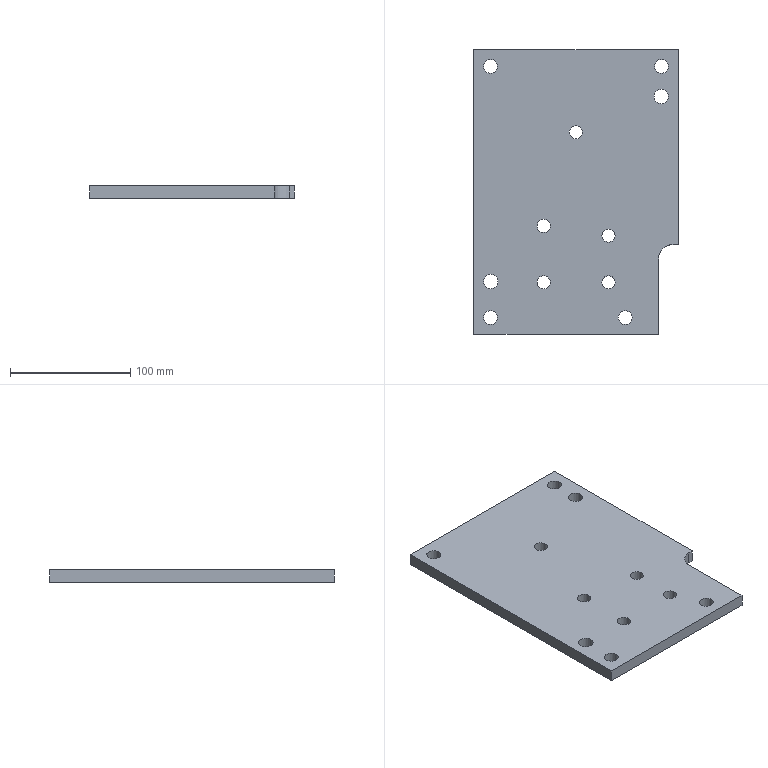Part | STEP file | lll_id2994_x_t | 1 solid | 20 faces | box 170 x 237 x 10 mm | volume 379901 mm3 | cylinder 12 | plane 8 | commonest cylinder face diameters 11 x5 11.509 x4 12 x2 24 x1
STEP:
#1=CARTESIAN_POINT('',(3581.734,202.95,92.5));
#2=VERTEX_POINT('',#1);
#3=CARTESIAN_POINT('',(3587.234,202.95,92.5));
#4=DIRECTION('',(0.,0.,-1.));
#5=DIRECTION('',(-1.,0.,0.));
#6=AXIS2_PLACEMENT_3D('',#3,#4,#5);
#7=CIRCLE('',#6,5.5);
#8=EDGE_CURVE('',#2,#2,#7,.T.);
#9=ORIENTED_EDGE('',*,*,#8,.F.);
#10=EDGE_LOOP('',(#9));
#11=FACE_BOUND('',#10,.T.);
#12=CARTESIAN_POINT('',(3608.779,117.031,92.5));
#13=VERTEX_POINT('',#12);
#14=CARTESIAN_POINT('',(3614.279,117.031,92.5));
#15=DIRECTION('',(0.,0.,-1.));
#16=DIRECTION('',(-1.,0.,0.));
#17=AXIS2_PLACEMENT_3D('',#14,#15,#16);
#18=CIRCLE('',#17,5.5);
#19=EDGE_CURVE('',#13,#13,#18,.T.);
#20=ORIENTED_EDGE('',*,*,#19,.F.);
#21=EDGE_LOOP('',(#20));
#22=FACE_BOUND('',#21,.T.);
#23=CARTESIAN_POINT('',(3554.876,78.05,92.5));
#24=VERTEX_POINT('',#23);
#25=CARTESIAN_POINT('',(3560.376,78.05,92.5));
#26=DIRECTION('',(0.,0.,-1.));
#27=DIRECTION('',(-1.,0.,0.));
#28=AXIS2_PLACEMENT_3D('',#25,#26,#27);
#29=CIRCLE('',#28,5.5);
#30=EDGE_CURVE('',#24,#24,#29,.T.);
#31=ORIENTED_EDGE('',*,*,#30,.F.);
#32=EDGE_LOOP('',(#31));
#33=FACE_BOUND('',#32,.T.);
#34=CARTESIAN_POINT('',(3510.243,78.803,92.5));
#35=VERTEX_POINT('',#34);
#36=CARTESIAN_POINT('',(3516.243,78.803,92.5));
#37=DIRECTION('',(0.,0.,1.));
#38=DIRECTION('',(-1.,0.,0.));
#39=AXIS2_PLACEMENT_3D('',#36,#37,#38);
#40=CIRCLE('',#39,6.);
#41=EDGE_CURVE('',#35,#35,#40,.T.);
#42=ORIENTED_EDGE('',*,*,#41,.T.);
#43=EDGE_LOOP('',(#42));
#44=FACE_BOUND('',#43,.T.);
#45=CARTESIAN_POINT('',(3622.489,48.803,92.5));
#46=VERTEX_POINT('',#45);
#47=CARTESIAN_POINT('',(3628.243,48.803,92.5));
#48=DIRECTION('',(0.,0.,1.));
#49=DIRECTION('',(-1.,0.,0.));
#50=AXIS2_PLACEMENT_3D('',#47,#48,#49);
#51=CIRCLE('',#50,5.755);
#52=EDGE_CURVE('',#46,#46,#51,.T.);
#53=ORIENTED_EDGE('',*,*,#52,.T.);
#54=EDGE_LOOP('',(#53));
#55=FACE_BOUND('',#54,.T.);
#56=CARTESIAN_POINT('',(3510.489,48.803,92.5));
#57=VERTEX_POINT('',#56);
#58=CARTESIAN_POINT('',(3516.243,48.803,92.5));
#59=DIRECTION('',(0.,0.,1.));
#60=DIRECTION('',(-1.,0.,0.));
#61=AXIS2_PLACEMENT_3D('',#58,#59,#60);
#62=CIRCLE('',#61,5.755);
#63=EDGE_CURVE('',#57,#57,#62,.T.);
#64=ORIENTED_EDGE('',*,*,#63,.T.);
#65=EDGE_LOOP('',(#64));
#66=FACE_BOUND('',#65,.T.);
#67=CARTESIAN_POINT('',(3652.489,257.803,92.5));
#68=VERTEX_POINT('',#67);
#69=CARTESIAN_POINT('',(3658.243,257.803,92.5));
#70=DIRECTION('',(0.,0.,1.));
#71=DIRECTION('',(-1.,0.,0.));
#72=AXIS2_PLACEMENT_3D('',#69,#70,#71);
#73=CIRCLE('',#72,5.755);
#74=EDGE_CURVE('',#68,#68,#73,.T.);
#75=ORIENTED_EDGE('',*,*,#74,.T.);
#76=EDGE_LOOP('',(#75));
#77=FACE_BOUND('',#76,.T.);
#78=CARTESIAN_POINT('',(3510.489,257.803,92.5));
#79=VERTEX_POINT('',#78);
#80=CARTESIAN_POINT('',(3516.243,257.803,92.5));
#81=DIRECTION('',(0.,0.,1.));
#82=DIRECTION('',(-1.,0.,0.));
#83=AXIS2_PLACEMENT_3D('',#80,#81,#82);
#84=CIRCLE('',#83,5.755);
#85=EDGE_CURVE('',#79,#79,#84,.T.);
#86=ORIENTED_EDGE('',*,*,#85,.T.);
#87=EDGE_LOOP('',(#86));
#88=FACE_BOUND('',#87,.T.);
#89=CARTESIAN_POINT('',(3652.243,232.803,92.5));
#90=VERTEX_POINT('',#89);
#91=CARTESIAN_POINT('',(3658.243,232.803,92.5));
#92=DIRECTION('',(0.,0.,1.));
#93=DIRECTION('',(-1.,0.,0.));
#94=AXIS2_PLACEMENT_3D('',#91,#92,#93);
#95=CIRCLE('',#94,6.);
#96=EDGE_CURVE('',#90,#90,#95,.T.);
#97=ORIENTED_EDGE('',*,*,#96,.T.);
#98=EDGE_LOOP('',(#97));
#99=FACE_BOUND('',#98,.T.);
#100=CARTESIAN_POINT('',(3672.243,109.5,92.5));
#101=VERTEX_POINT('',#100);
#102=CARTESIAN_POINT('',(3668.,109.5,92.5));
#103=VERTEX_POINT('',#102);
#104=CARTESIAN_POINT('',(3700.5,109.5,92.5));
#105=DIRECTION('',(-1.,0.,0.));
#106=VECTOR('',#105,1.);
#107=LINE('',#104,#106);
#108=EDGE_CURVE('',#101,#103,#107,.T.);
#109=ORIENTED_EDGE('',*,*,#108,.T.);
#110=CARTESIAN_POINT('',(3656.,97.5,92.5));
#111=VERTEX_POINT('',#110);
#112=CARTESIAN_POINT('',(3668.,97.5,92.5));
#113=DIRECTION('',(0.,0.,1.));
#114=DIRECTION('',(-1.,0.,0.));
#115=AXIS2_PLACEMENT_3D('',#112,#113,#114);
#116=CIRCLE('',#115,12.);
#117=EDGE_CURVE('',#103,#111,#116,.T.);
#118=ORIENTED_EDGE('',*,*,#117,.T.);
#119=CARTESIAN_POINT('',(3656.,34.803,92.5));
#120=VERTEX_POINT('',#119);
#121=CARTESIAN_POINT('',(3656.,0.00007612,92.5));
#122=DIRECTION('',(0.,-1.,0.));
#123=VECTOR('',#122,1.);
#124=LINE('',#121,#123);
#125=EDGE_CURVE('',#111,#120,#124,.T.);
#126=ORIENTED_EDGE('',*,*,#125,.T.);
#127=CARTESIAN_POINT('',(3502.243,34.803,92.5));
#128=VERTEX_POINT('',#127);
#129=CARTESIAN_POINT('',(3587.243,34.803,92.5));
#130=DIRECTION('',(1.,0.,0.));
#131=VECTOR('',#130,1.);
#132=LINE('',#129,#131);
#133=EDGE_CURVE('',#128,#120,#132,.T.);
#134=ORIENTED_EDGE('',*,*,#133,.F.);
#135=CARTESIAN_POINT('',(3502.243,271.803,92.5));
#136=VERTEX_POINT('',#135);
#137=CARTESIAN_POINT('',(3502.243,156.803,92.5));
#138=DIRECTION('',(0.,-1.,0.));
#139=VECTOR('',#138,1.);
#140=LINE('',#137,#139);
#141=EDGE_CURVE('',#136,#128,#140,.T.);
#142=ORIENTED_EDGE('',*,*,#141,.F.);
#143=CARTESIAN_POINT('',(3672.243,271.803,92.5));
#144=VERTEX_POINT('',#143);
#145=CARTESIAN_POINT('',(3587.243,271.803,92.5));
#146=DIRECTION('',(-1.,0.,0.));
#147=VECTOR('',#146,1.);
#148=LINE('',#145,#147);
#149=EDGE_CURVE('',#144,#136,#148,.T.);
#150=ORIENTED_EDGE('',*,*,#149,.F.);
#151=CARTESIAN_POINT('',(3672.243,156.803,92.5));
#152=DIRECTION('',(0.,1.,0.));
#153=VECTOR('',#152,1.);
#154=LINE('',#151,#153);
#155=EDGE_CURVE('',#101,#144,#154,.T.);
#156=ORIENTED_EDGE('',*,*,#155,.F.);
#157=EDGE_LOOP('',(#109,#118,#126,#134,#142,#150,#156));
#158=FACE_BOUND('',#157,.T.);
#159=CARTESIAN_POINT('',(3608.779,78.031,92.5));
#160=VERTEX_POINT('',#159);
#161=CARTESIAN_POINT('',(3614.279,78.031,92.5));
#162=DIRECTION('',(0.,0.,-1.));
#163=DIRECTION('',(-1.,0.,0.));
#164=AXIS2_PLACEMENT_3D('',#161,#162,#163);
#165=CIRCLE('',#164,5.5);
#166=EDGE_CURVE('',#160,#160,#165,.T.);
#167=ORIENTED_EDGE('',*,*,#166,.F.);
#168=EDGE_LOOP('',(#167));
#169=FACE_BOUND('',#168,.T.);
#170=CARTESIAN_POINT('',(3554.876,125.05,92.5));
#171=VERTEX_POINT('',#170);
#172=CARTESIAN_POINT('',(3560.376,125.05,92.5));
#173=DIRECTION('',(0.,0.,1.));
#174=DIRECTION('',(-1.,0.,0.));
#175=AXIS2_PLACEMENT_3D('',#172,#173,#174);
#176=CIRCLE('',#175,5.5);
#177=EDGE_CURVE('',#171,#171,#176,.T.);
#178=ORIENTED_EDGE('',*,*,#177,.T.);
#179=EDGE_LOOP('',(#178));
#180=FACE_BOUND('',#179,.T.);
#181=CARTESIAN_POINT('',(3587.243,156.803,92.5));
#182=DIRECTION('',(0.,0.,-1.));
#183=DIRECTION('',(1.,0.,0.));
#184=AXIS2_PLACEMENT_3D('',#181,#182,#183);
#185=PLANE('',#184);
#186=ADVANCED_FACE('',(#11,#22,#33,#44,#55,#66,#77,#88,#99,#158,#169,#180),#185,.T.);
#187=CARTESIAN_POINT('',(3581.734,202.95,102.5));
#188=VERTEX_POINT('',#187);
#189=CARTESIAN_POINT('',(3587.234,202.95,102.5));
#190=DIRECTION('',(0.,0.,-1.));
#191=DIRECTION('',(-1.,0.,0.));
#192=AXIS2_PLACEMENT_3D('',#189,#190,#191);
#193=CIRCLE('',#192,5.5);
#194=EDGE_CURVE('',#188,#188,#193,.T.);
#195=ORIENTED_EDGE('',*,*,#194,.T.);
#196=EDGE_LOOP('',(#195));
#197=FACE_BOUND('',#196,.T.);
#198=CARTESIAN_POINT('',(3608.779,117.031,102.5));
#199=VERTEX_POINT('',#198);
#200=CARTESIAN_POINT('',(3614.279,117.031,102.5));
#201=DIRECTION('',(0.,0.,-1.));
#202=DIRECTION('',(-1.,0.,0.));
#203=AXIS2_PLACEMENT_3D('',#200,#201,#202);
#204=CIRCLE('',#203,5.5);
#205=EDGE_CURVE('',#199,#199,#204,.T.);
#206=ORIENTED_EDGE('',*,*,#205,.T.);
#207=EDGE_LOOP('',(#206));
#208=FACE_BOUND('',#207,.T.);
#209=CARTESIAN_POINT('',(3554.876,78.05,102.5));
#210=VERTEX_POINT('',#209);
#211=CARTESIAN_POINT('',(3560.376,78.05,102.5));
#212=DIRECTION('',(0.,0.,-1.));
#213=DIRECTION('',(-1.,0.,0.));
#214=AXIS2_PLACEMENT_3D('',#211,#212,#213);
#215=CIRCLE('',#214,5.5);
#216=EDGE_CURVE('',#210,#210,#215,.T.);
#217=ORIENTED_EDGE('',*,*,#216,.T.);
#218=EDGE_LOOP('',(#217));
#219=FACE_BOUND('',#218,.T.);
#220=CARTESIAN_POINT('',(3652.489,257.803,102.5));
#221=VERTEX_POINT('',#220);
#222=CARTESIAN_POINT('',(3658.243,257.803,102.5));
#223=DIRECTION('',(0.,0.,1.));
#224=DIRECTION('',(-1.,0.,0.));
#225=AXIS2_PLACEMENT_3D('',#222,#223,#224);
#226=CIRCLE('',#225,5.755);
#227=EDGE_CURVE('',#221,#221,#226,.T.);
#228=ORIENTED_EDGE('',*,*,#227,.F.);
#229=EDGE_LOOP('',(#228));
#230=FACE_BOUND('',#229,.T.);
#231=CARTESIAN_POINT('',(3510.489,257.803,102.5));
#232=VERTEX_POINT('',#231);
#233=CARTESIAN_POINT('',(3516.243,257.803,102.5));
#234=DIRECTION('',(0.,0.,-1.));
#235=DIRECTION('',(-1.,0.,0.));
#236=AXIS2_PLACEMENT_3D('',#233,#234,#235);
#237=CIRCLE('',#236,5.755);
#238=EDGE_CURVE('',#232,#232,#237,.T.);
#239=ORIENTED_EDGE('',*,*,#238,.T.);
#240=EDGE_LOOP('',(#239));
#241=FACE_BOUND('',#240,.T.);
#242=CARTESIAN_POINT('',(3652.243,232.803,102.5));
#243=VERTEX_POINT('',#242);
#244=CARTESIAN_POINT('',(3658.243,232.803,102.5));
#245=DIRECTION('',(0.,0.,-1.));
#246=DIRECTION('',(-1.,0.,0.));
#247=AXIS2_PLACEMENT_3D('',#244,#245,#246);
#248=CIRCLE('',#247,6.);
#249=EDGE_CURVE('',#243,#243,#248,.T.);
#250=ORIENTED_EDGE('',*,*,#249,.T.);
#251=EDGE_LOOP('',(#250));
#252=FACE_BOUND('',#251,.T.);
#253=CARTESIAN_POINT('',(3502.243,271.803,102.5));
#254=VERTEX_POINT('',#253);
#255=CARTESIAN_POINT('',(3672.243,271.803,102.5));
#256=VERTEX_POINT('',#255);
#257=CARTESIAN_POINT('',(3587.243,271.803,102.5));
#258=DIRECTION('',(1.,0.,0.));
#259=VECTOR('',#258,1.);
#260=LINE('',#257,#259);
#261=EDGE_CURVE('',#254,#256,#260,.T.);
#262=ORIENTED_EDGE('',*,*,#261,.F.);
#263=CARTESIAN_POINT('',(3502.243,34.803,102.5));
#264=VERTEX_POINT('',#263);
#265=CARTESIAN_POINT('',(3502.243,156.803,102.5));
#266=DIRECTION('',(0.,1.,0.));
#267=VECTOR('',#266,1.);
#268=LINE('',#265,#267);
#269=EDGE_CURVE('',#264,#254,#268,.T.);
#270=ORIENTED_EDGE('',*,*,#269,.F.);
#271=CARTESIAN_POINT('',(3656.,34.803,102.5));
#272=VERTEX_POINT('',#271);
#273=CARTESIAN_POINT('',(3587.243,34.803,102.5));
#274=DIRECTION('',(-1.,0.,0.));
#275=VECTOR('',#274,1.);
#276=LINE('',#273,#275);
#277=EDGE_CURVE('',#272,#264,#276,.T.);
#278=ORIENTED_EDGE('',*,*,#277,.F.);
#279=CARTESIAN_POINT('',(3656.,97.5,102.5));
#280=VERTEX_POINT('',#279);
#281=CARTESIAN_POINT('',(3656.,136.288,102.5));
#282=DIRECTION('',(0.,1.,0.));
#283=VECTOR('',#282,1.);
#284=LINE('',#281,#283);
#285=EDGE_CURVE('',#272,#280,#284,.T.);
#286=ORIENTED_EDGE('',*,*,#285,.T.);
#287=CARTESIAN_POINT('',(3668.,109.5,102.5));
#288=VERTEX_POINT('',#287);
#289=CARTESIAN_POINT('',(3668.,97.5,102.5));
#290=DIRECTION('',(0.,0.,1.));
#291=DIRECTION('',(-1.,0.,0.));
#292=AXIS2_PLACEMENT_3D('',#289,#290,#291);
#293=CIRCLE('',#292,12.);
#294=EDGE_CURVE('',#288,#280,#293,.T.);
#295=ORIENTED_EDGE('',*,*,#294,.F.);
#296=CARTESIAN_POINT('',(3672.243,109.5,102.5));
#297=VERTEX_POINT('',#296);
#298=CARTESIAN_POINT('',(3312.867,109.5,102.5));
#299=DIRECTION('',(1.,0.,0.));
#300=VECTOR('',#299,1.);
#301=LINE('',#298,#300);
#302=EDGE_CURVE('',#288,#297,#301,.T.);
#303=ORIENTED_EDGE('',*,*,#302,.T.);
#304=CARTESIAN_POINT('',(3672.243,156.803,102.5));
#305=DIRECTION('',(0.,-1.,0.));
#306=VECTOR('',#305,1.);
#307=LINE('',#304,#306);
#308=EDGE_CURVE('',#256,#297,#307,.T.);
#309=ORIENTED_EDGE('',*,*,#308,.F.);
#310=EDGE_LOOP('',(#262,#270,#278,#286,#295,#303,#309));
#311=FACE_BOUND('',#310,.T.);
#312=CARTESIAN_POINT('',(3510.243,78.803,102.5));
#313=VERTEX_POINT('',#312);
#314=CARTESIAN_POINT('',(3516.243,78.803,102.5));
#315=DIRECTION('',(0.,0.,1.));
#316=DIRECTION('',(-1.,0.,0.));
#317=AXIS2_PLACEMENT_3D('',#314,#315,#316);
#318=CIRCLE('',#317,6.);
#319=EDGE_CURVE('',#313,#313,#318,.T.);
#320=ORIENTED_EDGE('',*,*,#319,.F.);
#321=EDGE_LOOP('',(#320));
#322=FACE_BOUND('',#321,.T.);
#323=CARTESIAN_POINT('',(3622.489,48.803,102.5));
#324=VERTEX_POINT('',#323);
#325=CARTESIAN_POINT('',(3628.243,48.803,102.5));
#326=DIRECTION('',(0.,0.,1.));
#327=DIRECTION('',(-1.,0.,0.));
#328=AXIS2_PLACEMENT_3D('',#325,#326,#327);
#329=CIRCLE('',#328,5.755);
#330=EDGE_CURVE('',#324,#324,#329,.T.);
#331=ORIENTED_EDGE('',*,*,#330,.F.);
#332=EDGE_LOOP('',(#331));
#333=FACE_BOUND('',#332,.T.);
#334=CARTESIAN_POINT('',(3510.489,48.803,102.5));
#335=VERTEX_POINT('',#334);
#336=CARTESIAN_POINT('',(3516.243,48.803,102.5));
#337=DIRECTION('',(0.,0.,1.));
#338=DIRECTION('',(-1.,0.,0.));
#339=AXIS2_PLACEMENT_3D('',#336,#337,#338);
#340=CIRCLE('',#339,5.755);
#341=EDGE_CURVE('',#335,#335,#340,.T.);
#342=ORIENTED_EDGE('',*,*,#341,.F.);
#343=EDGE_LOOP('',(#342));
#344=FACE_BOUND('',#343,.T.);
#345=CARTESIAN_POINT('',(3608.779,78.031,102.5));
#346=VERTEX_POINT('',#345);
#347=CARTESIAN_POINT('',(3614.279,78.031,102.5));
#348=DIRECTION('',(0.,0.,-1.));
#349=DIRECTION('',(-1.,0.,0.));
#350=AXIS2_PLACEMENT_3D('',#347,#348,#349);
#351=CIRCLE('',#350,5.5);
#352=EDGE_CURVE('',#346,#346,#351,.T.);
#353=ORIENTED_EDGE('',*,*,#352,.T.);
#354=EDGE_LOOP('',(#353));
#355=FACE_BOUND('',#354,.T.);
#356=CARTESIAN_POINT('',(3554.876,125.05,102.5));
#357=VERTEX_POINT('',#356);
#358=CARTESIAN_POINT('',(3560.376,125.05,102.5));
#359=DIRECTION('',(0.,0.,1.));
#360=DIRECTION('',(-1.,0.,0.));
#361=AXIS2_PLACEMENT_3D('',#358,#359,#360);
#362=CIRCLE('',#361,5.5);
#363=EDGE_CURVE('',#357,#357,#362,.T.);
#364=ORIENTED_EDGE('',*,*,#363,.F.);
#365=EDGE_LOOP('',(#364));
#366=FACE_BOUND('',#365,.T.);
#367=CARTESIAN_POINT('',(3312.867,136.288,102.5));
#368=DIRECTION('',(0.,0.,-1.));
#369=DIRECTION('',(-1.,0.,0.));
#370=AXIS2_PLACEMENT_3D('',#367,#368,#369);
#371=PLANE('',#370);
#372=ADVANCED_FACE('',(#197,#208,#219,#230,#241,#252,#311,#322,#333,#344,#355,#366),#371,.F.);
#373=ORIENTED_EDGE('',*,*,#319,.T.);
#374=EDGE_LOOP('',(#373));
#375=FACE_BOUND('',#374,.T.);
#376=ORIENTED_EDGE('',*,*,#41,.F.);
#377=EDGE_LOOP('',(#376));
#378=FACE_BOUND('',#377,.T.);
#379=CARTESIAN_POINT('',(3516.243,78.803,92.5));
#380=DIRECTION('',(0.,0.,1.));
#381=DIRECTION('',(-1.,0.,0.));
#382=AXIS2_PLACEMENT_3D('',#379,#380,#381);
#383=CYLINDRICAL_SURFACE('',#382,6.);
#384=ADVANCED_FACE('',(#375,#378),#383,.F.);
#385=ORIENTED_EDGE('',*,*,#330,.T.);
#386=EDGE_LOOP('',(#385));
#387=FACE_BOUND('',#386,.T.);
#388=ORIENTED_EDGE('',*,*,#52,.F.);
#389=EDGE_LOOP('',(#388));
#390=FACE_BOUND('',#389,.T.);
#391=CARTESIAN_POINT('',(3628.243,48.803,92.5));
#392=DIRECTION('',(0.,0.,1.));
#393=DIRECTION('',(-1.,0.,0.));
#394=AXIS2_PLACEMENT_3D('',#391,#392,#393);
#395=CYLINDRICAL_SURFACE('',#394,5.755);
#396=ADVANCED_FACE('',(#387,#390),#395,.F.);
#397=ORIENTED_EDGE('',*,*,#341,.T.);
#398=EDGE_LOOP('',(#397));
#399=FACE_BOUND('',#398,.T.);
#400=ORIENTED_EDGE('',*,*,#63,.F.);
#401=EDGE_LOOP('',(#400));
#402=FACE_BOUND('',#401,.T.);
#403=CARTESIAN_POINT('',(3516.243,48.803,92.5));
#404=DIRECTION('',(0.,0.,1.));
#405=DIRECTION('',(-1.,0.,0.));
#406=AXIS2_PLACEMENT_3D('',#403,#404,#405);
#407=CYLINDRICAL_SURFACE('',#406,5.755);
#408=ADVANCED_FACE('',(#399,#402),#407,.F.);
#409=ORIENTED_EDGE('',*,*,#227,.T.);
#410=EDGE_LOOP('',(#409));
#411=FACE_BOUND('',#410,.T.);
#412=ORIENTED_EDGE('',*,*,#74,.F.);
#413=EDGE_LOOP('',(#412));
#414=FACE_BOUND('',#413,.T.);
#415=CARTESIAN_POINT('',(3658.243,257.803,92.5));
#416=DIRECTION('',(0.,0.,1.));
#417=DIRECTION('',(-1.,0.,0.));
#418=AXIS2_PLACEMENT_3D('',#415,#416,#417);
#419=CYLINDRICAL_SURFACE('',#418,5.755);
#420=ADVANCED_FACE('',(#411,#414),#419,.F.);
#421=ORIENTED_EDGE('',*,*,#238,.F.);
#422=EDGE_LOOP('',(#421));
#423=FACE_BOUND('',#422,.T.);
#424=ORIENTED_EDGE('',*,*,#85,.F.);
#425=EDGE_LOOP('',(#424));
#426=FACE_BOUND('',#425,.T.);
#427=CARTESIAN_POINT('',(3516.243,257.803,92.5));
#428=DIRECTION('',(0.,0.,1.));
#429=DIRECTION('',(-1.,0.,0.));
#430=AXIS2_PLACEMENT_3D('',#427,#428,#429);
#431=CYLINDRICAL_SURFACE('',#430,5.755);
#432=ADVANCED_FACE('',(#423,#426),#431,.F.);
#433=ORIENTED_EDGE('',*,*,#249,.F.);
#434=EDGE_LOOP('',(#433));
#435=FACE_BOUND('',#434,.T.);
#436=ORIENTED_EDGE('',*,*,#96,.F.);
#437=EDGE_LOOP('',(#436));
#438=FACE_BOUND('',#437,.T.);
#439=CARTESIAN_POINT('',(3658.243,232.803,92.5));
#440=DIRECTION('',(0.,0.,1.));
#441=DIRECTION('',(-1.,0.,0.));
#442=AXIS2_PLACEMENT_3D('',#439,#440,#441);
#443=CYLINDRICAL_SURFACE('',#442,6.);
#444=ADVANCED_FACE('',(#435,#438),#443,.F.);
#445=CARTESIAN_POINT('',(3668.,109.5,92.5));
#446=DIRECTION('',(0.,0.,-1.));
#447=VECTOR('',#446,1.);
#448=LINE('',#445,#447);
#449=EDGE_CURVE('',#288,#103,#448,.T.);
#450=ORIENTED_EDGE('',*,*,#449,.F.);
#451=ORIENTED_EDGE('',*,*,#294,.T.);
#452=CARTESIAN_POINT('',(3656.,97.5,92.5));
#453=DIRECTION('',(0.,0.,1.));
#454=VECTOR('',#453,1.);
#455=LINE('',#452,#454);
#456=EDGE_CURVE('',#111,#280,#455,.T.);
#457=ORIENTED_EDGE('',*,*,#456,.F.);
#458=ORIENTED_EDGE('',*,*,#117,.F.);
#459=EDGE_LOOP('',(#450,#451,#457,#458));
#460=FACE_OUTER_BOUND('',#459,.T.);
#461=CARTESIAN_POINT('',(3668.,97.5,92.5));
#462=DIRECTION('',(0.,0.,1.));
#463=DIRECTION('',(1.,0.,0.));
#464=AXIS2_PLACEMENT_3D('',#461,#462,#463);
#465=CYLINDRICAL_SURFACE('',#464,12.);
#466=ADVANCED_FACE('',(#460),#465,.F.);
#467=CARTESIAN_POINT('',(3672.243,109.5,92.5));
#468=DIRECTION('',(0.,0.,1.));
#469=VECTOR('',#468,1.);
#470=LINE('',#467,#469);
#471=EDGE_CURVE('',#101,#297,#470,.T.);
#472=ORIENTED_EDGE('',*,*,#471,.T.);
#473=ORIENTED_EDGE('',*,*,#302,.F.);
#474=ORIENTED_EDGE('',*,*,#449,.T.);
#475=ORIENTED_EDGE('',*,*,#108,.F.);
#476=EDGE_LOOP('',(#472,#473,#474,#475));
#477=FACE_OUTER_BOUND('',#476,.T.);
#478=CARTESIAN_POINT('',(3700.5,109.5,92.5));
#479=DIRECTION('',(0.,1.,0.));
#480=DIRECTION('',(0.,0.,-1.));
#481=AXIS2_PLACEMENT_3D('',#478,#479,#480);
#482=PLANE('',#481);
#483=ADVANCED_FACE('',(#477),#482,.F.);
#484=ORIENTED_EDGE('',*,*,#456,.T.);
#485=ORIENTED_EDGE('',*,*,#285,.F.);
#486=CARTESIAN_POINT('',(3656.,34.803,92.5));
#487=DIRECTION('',(0.,0.,-1.));
#488=VECTOR('',#487,1.);
#489=LINE('',#486,#488);
#490=EDGE_CURVE('',#272,#120,#489,.T.);
#491=ORIENTED_EDGE('',*,*,#490,.T.);
#492=ORIENTED_EDGE('',*,*,#125,.F.);
#493=EDGE_LOOP('',(#484,#485,#491,#492));
#494=FACE_OUTER_BOUND('',#493,.T.);
#495=CARTESIAN_POINT('',(3656.,0.00007612,92.5));
#496=DIRECTION('',(-1.,0.,0.));
#497=DIRECTION('',(0.,0.,-1.));
#498=AXIS2_PLACEMENT_3D('',#495,#496,#497);
#499=PLANE('',#498);
#500=ADVANCED_FACE('',(#494),#499,.F.);
#501=ORIENTED_EDGE('',*,*,#269,.T.);
#502=CARTESIAN_POINT('',(3502.243,271.803,92.5));
#503=DIRECTION('',(0.,0.,1.));
#504=VECTOR('',#503,1.);
#505=LINE('',#502,#504);
#506=EDGE_CURVE('',#136,#254,#505,.T.);
#507=ORIENTED_EDGE('',*,*,#506,.F.);
#508=ORIENTED_EDGE('',*,*,#141,.T.);
#509=CARTESIAN_POINT('',(3502.243,34.803,92.5));
#510=DIRECTION('',(0.,0.,1.));
#511=VECTOR('',#510,1.);
#512=LINE('',#509,#511);
#513=EDGE_CURVE('',#128,#264,#512,.T.);
#514=ORIENTED_EDGE('',*,*,#513,.T.);
#515=EDGE_LOOP('',(#501,#507,#508,#514));
#516=FACE_OUTER_BOUND('',#515,.T.);
#517=CARTESIAN_POINT('',(3502.243,156.803,92.5));
#518=DIRECTION('',(-1.,0.,0.));
#519=DIRECTION('',(0.,0.,-1.));
#520=AXIS2_PLACEMENT_3D('',#517,#518,#519);
#521=PLANE('',#520);
#522=ADVANCED_FACE('',(#516),#521,.T.);
#523=ORIENTED_EDGE('',*,*,#277,.T.);
#524=ORIENTED_EDGE('',*,*,#513,.F.);
#525=ORIENTED_EDGE('',*,*,#133,.T.);
#526=ORIENTED_EDGE('',*,*,#490,.F.);
#527=EDGE_LOOP('',(#523,#524,#525,#526));
#528=FACE_OUTER_BOUND('',#527,.T.);
#529=CARTESIAN_POINT('',(3587.243,34.803,92.5));
#530=DIRECTION('',(0.,-1.,0.));
#531=DIRECTION('',(0.,0.,1.));
#532=AXIS2_PLACEMENT_3D('',#529,#530,#531);
#533=PLANE('',#532);
#534=ADVANCED_FACE('',(#528),#533,.T.);
#535=ORIENTED_EDGE('',*,*,#261,.T.);
#536=CARTESIAN_POINT('',(3672.243,271.803,92.5));
#537=DIRECTION('',(0.,0.,1.));
#538=VECTOR('',#537,1.);
#539=LINE('',#536,#538);
#540=EDGE_CURVE('',#144,#256,#539,.T.);
#541=ORIENTED_EDGE('',*,*,#540,.F.);
#542=ORIENTED_EDGE('',*,*,#149,.T.);
#543=ORIENTED_EDGE('',*,*,#506,.T.);
#544=EDGE_LOOP('',(#535,#541,#542,#543));
#545=FACE_OUTER_BOUND('',#544,.T.);
#546=CARTESIAN_POINT('',(3587.243,271.803,92.5));
#547=DIRECTION('',(0.,1.,0.));
#548=DIRECTION('',(0.,0.,-1.));
#549=AXIS2_PLACEMENT_3D('',#546,#547,#548);
#550=PLANE('',#549);
#551=ADVANCED_FACE('',(#545),#550,.T.);
#552=ORIENTED_EDGE('',*,*,#308,.T.);
#553=ORIENTED_EDGE('',*,*,#471,.F.);
#554=ORIENTED_EDGE('',*,*,#155,.T.);
#555=ORIENTED_EDGE('',*,*,#540,.T.);
#556=EDGE_LOOP('',(#552,#553,#554,#555));
#557=FACE_OUTER_BOUND('',#556,.T.);
#558=CARTESIAN_POINT('',(3672.243,156.803,92.5));
#559=DIRECTION('',(1.,0.,0.));
#560=DIRECTION('',(0.,0.,1.));
#561=AXIS2_PLACEMENT_3D('',#558,#559,#560);
#562=PLANE('',#561);
#563=ADVANCED_FACE('',(#557),#562,.T.);
#564=ORIENTED_EDGE('',*,*,#166,.T.);
#565=EDGE_LOOP('',(#564));
#566=FACE_BOUND('',#565,.T.);
#567=ORIENTED_EDGE('',*,*,#352,.F.);
#568=EDGE_LOOP('',(#567));
#569=FACE_BOUND('',#568,.T.);
#570=CARTESIAN_POINT('',(3614.279,78.031,212.5));
#571=DIRECTION('',(0.,0.,-1.));
#572=DIRECTION('',(-1.,0.,0.));
#573=AXIS2_PLACEMENT_3D('',#570,#571,#572);
#574=CYLINDRICAL_SURFACE('',#573,5.5);
#575=ADVANCED_FACE('',(#566,#569),#574,.F.);
#576=ORIENTED_EDGE('',*,*,#177,.F.);
#577=EDGE_LOOP('',(#576));
#578=FACE_BOUND('',#577,.T.);
#579=ORIENTED_EDGE('',*,*,#363,.T.);
#580=EDGE_LOOP('',(#579));
#581=FACE_BOUND('',#580,.T.);
#582=CARTESIAN_POINT('',(3560.376,125.05,212.5));
#583=DIRECTION('',(0.,0.,-1.));
#584=DIRECTION('',(-1.,0.,0.));
#585=AXIS2_PLACEMENT_3D('',#582,#583,#584);
#586=CYLINDRICAL_SURFACE('',#585,5.5);
#587=ADVANCED_FACE('',(#578,#581),#586,.F.);
#588=ORIENTED_EDGE('',*,*,#30,.T.);
#589=EDGE_LOOP('',(#588));
#590=FACE_BOUND('',#589,.T.);
#591=ORIENTED_EDGE('',*,*,#216,.F.);
#592=EDGE_LOOP('',(#591));
#593=FACE_BOUND('',#592,.T.);
#594=CARTESIAN_POINT('',(3560.376,78.05,212.5));
#595=DIRECTION('',(0.,0.,-1.));
#596=DIRECTION('',(-1.,0.,0.));
#597=AXIS2_PLACEMENT_3D('',#594,#595,#596);
#598=CYLINDRICAL_SURFACE('',#597,5.5);
#599=ADVANCED_FACE('',(#590,#593),#598,.F.);
#600=ORIENTED_EDGE('',*,*,#19,.T.);
#601=EDGE_LOOP('',(#600));
#602=FACE_BOUND('',#601,.T.);
#603=ORIENTED_EDGE('',*,*,#205,.F.);
#604=EDGE_LOOP('',(#603));
#605=FACE_BOUND('',#604,.T.);
#606=CARTESIAN_POINT('',(3614.279,117.031,212.5));
#607=DIRECTION('',(0.,0.,-1.));
#608=DIRECTION('',(-1.,0.,0.));
#609=AXIS2_PLACEMENT_3D('',#606,#607,#608);
#610=CYLINDRICAL_SURFACE('',#609,5.5);
#611=ADVANCED_FACE('',(#602,#605),#610,.F.);
#612=ORIENTED_EDGE('',*,*,#8,.T.);
#613=EDGE_LOOP('',(#612));
#614=FACE_BOUND('',#613,.T.);
#615=ORIENTED_EDGE('',*,*,#194,.F.);
#616=EDGE_LOOP('',(#615));
#617=FACE_BOUND('',#616,.T.);
#618=CARTESIAN_POINT('',(3587.234,202.95,77.5));
#619=DIRECTION('',(0.,0.,1.));
#620=DIRECTION('',(-1.,0.,0.));
#621=AXIS2_PLACEMENT_3D('',#618,#619,#620);
#622=CYLINDRICAL_SURFACE('',#621,5.5);
#623=ADVANCED_FACE('',(#614,#617),#622,.F.);
#624=CLOSED_SHELL('',(#186,#372,#384,#396,#408,#420,#432,#444,#466,#483,#500,#522,#534,#551,#563,#575,#587,#599,#611,#623));
#625=MANIFOLD_SOLID_BREP('',#624);
#626=(LENGTH_UNIT()NAMED_UNIT(*)SI_UNIT(.MILLI.,.METRE.));
#627=UNCERTAINTY_MEASURE_WITH_UNIT(LENGTH_MEASURE(0.00002),#626,'','');
#628=(NAMED_UNIT(*)PLANE_ANGLE_UNIT()SI_UNIT($,.RADIAN.));
#629=PLANE_ANGLE_MEASURE_WITH_UNIT(PLANE_ANGLE_MEASURE(0.01745),#628);
#630=DIMENSIONAL_EXPONENTS(0.,0.,0.,0.,0.,0.,0.);
#631=(CONVERSION_BASED_UNIT('DEGREE',#629)NAMED_UNIT(#630)PLANE_ANGLE_UNIT());
#632=(NAMED_UNIT(*)SI_UNIT($,.STERADIAN.)SOLID_ANGLE_UNIT());
#633=(GEOMETRIC_REPRESENTATION_CONTEXT(3)GLOBAL_UNCERTAINTY_ASSIGNED_CONTEXT((#627))GLOBAL_UNIT_ASSIGNED_CONTEXT((#626,#631,#632))REPRESENTATION_CONTEXT('',''));
#634=ADVANCED_BREP_SHAPE_REPRESENTATION('',(#625),#633);